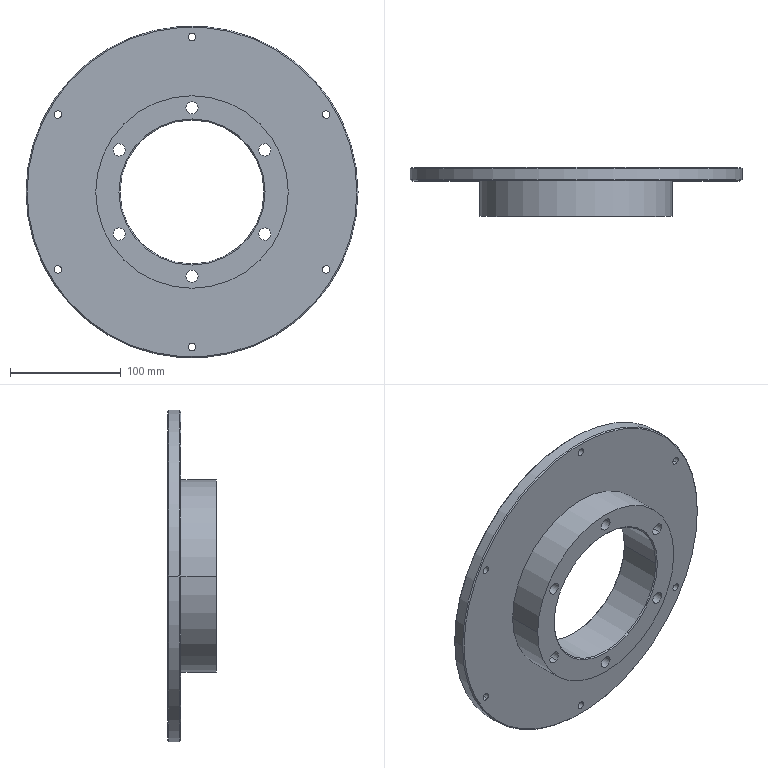Part | Creo | features CURVE 7, CUT 6, DATUM PLANE 3, PATTERN 2, CHAMFER 1, COORDINATE SYSTEM 1, PROTRUSION 1 | 1 solid | 44 faces | box 300 x 44 x 300 mm | volume 925584 mm3 | cylinder 32 | cone 8 | plane 4 | commonest cylinder face diameters 6.8 x12 11 x12 130 x2 174 x2 250 x2 300 x2
STEP:
#1=CARTESIAN_POINT('',(0.,0.,0.));
#2=DIRECTION('',(0.,0.,1.));
#3=DIRECTION('',(1.,0.,0.));
#4=AXIS2_PLACEMENT_3D('',#1,#2,#3);
#5=CARTESIAN_POINT('',(87.,0.,0.));
#6=VERTEX_POINT('',#5);
#7=CARTESIAN_POINT('',(-87.,0.,0.));
#8=VERTEX_POINT('',#7);
#9=CARTESIAN_POINT('',(0.,0.,0.));
#10=DIRECTION('',(0.,-1.,0.));
#11=DIRECTION('',(1.,0.,0.));
#12=AXIS2_PLACEMENT_3D('',#9,#10,#11);
#13=CIRCLE('',#12,87.);
#14=EDGE_CURVE('',#6,#8,#13,.T.);
#15=ORIENTED_EDGE('',*,*,#14,.F.);
#16=CARTESIAN_POINT('',(0.,0.,0.));
#17=DIRECTION('',(0.,1.,0.));
#18=DIRECTION('',(1.,0.,0.));
#19=AXIS2_PLACEMENT_3D('',#16,#17,#18);
#20=CIRCLE('',#19,87.);
#21=EDGE_CURVE('',#6,#8,#20,.T.);
#22=ORIENTED_EDGE('',*,*,#21,.T.);
#23=EDGE_LOOP('',(#15,#22));
#24=FACE_OUTER_BOUND('',#23,.F.);
#25=CARTESIAN_POINT('',(5.5,0.,-76.));
#26=VERTEX_POINT('',#25);
#27=CARTESIAN_POINT('',(-5.5,0.,-76.));
#28=VERTEX_POINT('',#27);
#29=CARTESIAN_POINT('',(0.,0.,-76.));
#30=DIRECTION('',(0.,1.,0.));
#31=DIRECTION('',(1.,0.,0.));
#32=AXIS2_PLACEMENT_3D('',#29,#30,#31);
#33=CIRCLE('',#32,5.5);
#34=EDGE_CURVE('',#26,#28,#33,.T.);
#35=ORIENTED_EDGE('',*,*,#34,.F.);
#36=CARTESIAN_POINT('',(0.,0.,-76.));
#37=DIRECTION('',(0.,1.,0.));
#38=DIRECTION('',(-1.,0.,0.));
#39=AXIS2_PLACEMENT_3D('',#36,#37,#38);
#40=CIRCLE('',#39,5.5);
#41=EDGE_CURVE('',#28,#26,#40,.T.);
#42=ORIENTED_EDGE('',*,*,#41,.F.);
#43=EDGE_LOOP('',(#35,#42));
#44=FACE_BOUND('',#43,.F.);
#45=CARTESIAN_POINT('',(-63.068,0.,-42.763));
#46=VERTEX_POINT('',#45);
#47=CARTESIAN_POINT('',(-68.568,0.,-33.237));
#48=VERTEX_POINT('',#47);
#49=CARTESIAN_POINT('',(-65.818,0.,-38.));
#50=DIRECTION('',(0.,1.,0.));
#51=DIRECTION('',(0.5,0.,-0.866));
#52=AXIS2_PLACEMENT_3D('',#49,#50,#51);
#53=CIRCLE('',#52,5.5);
#54=EDGE_CURVE('',#46,#48,#53,.T.);
#55=ORIENTED_EDGE('',*,*,#54,.F.);
#56=CARTESIAN_POINT('',(-65.818,0.,-38.));
#57=DIRECTION('',(0.,1.,0.));
#58=DIRECTION('',(-0.5,0.,0.866));
#59=AXIS2_PLACEMENT_3D('',#56,#57,#58);
#60=CIRCLE('',#59,5.5);
#61=EDGE_CURVE('',#48,#46,#60,.T.);
#62=ORIENTED_EDGE('',*,*,#61,.F.);
#63=EDGE_LOOP('',(#55,#62));
#64=FACE_BOUND('',#63,.F.);
#65=CARTESIAN_POINT('',(-68.568,0.,33.237));
#66=VERTEX_POINT('',#65);
#67=CARTESIAN_POINT('',(-63.068,0.,42.763));
#68=VERTEX_POINT('',#67);
#69=CARTESIAN_POINT('',(-65.818,0.,38.));
#70=DIRECTION('',(0.,1.,0.));
#71=DIRECTION('',(-0.5,0.,-0.866));
#72=AXIS2_PLACEMENT_3D('',#69,#70,#71);
#73=CIRCLE('',#72,5.5);
#74=EDGE_CURVE('',#66,#68,#73,.T.);
#75=ORIENTED_EDGE('',*,*,#74,.F.);
#76=CARTESIAN_POINT('',(-65.818,0.,38.));
#77=DIRECTION('',(0.,1.,0.));
#78=DIRECTION('',(0.5,0.,0.866));
#79=AXIS2_PLACEMENT_3D('',#76,#77,#78);
#80=CIRCLE('',#79,5.5);
#81=EDGE_CURVE('',#68,#66,#80,.T.);
#82=ORIENTED_EDGE('',*,*,#81,.F.);
#83=EDGE_LOOP('',(#75,#82));
#84=FACE_BOUND('',#83,.F.);
#85=CARTESIAN_POINT('',(-5.5,0.,76.));
#86=VERTEX_POINT('',#85);
#87=CARTESIAN_POINT('',(5.5,0.,76.));
#88=VERTEX_POINT('',#87);
#89=CARTESIAN_POINT('',(0.,0.,76.));
#90=DIRECTION('',(0.,1.,0.));
#91=DIRECTION('',(-1.,0.,0.));
#92=AXIS2_PLACEMENT_3D('',#89,#90,#91);
#93=CIRCLE('',#92,5.5);
#94=EDGE_CURVE('',#86,#88,#93,.T.);
#95=ORIENTED_EDGE('',*,*,#94,.F.);
#96=CARTESIAN_POINT('',(0.,0.,76.));
#97=DIRECTION('',(0.,1.,0.));
#98=DIRECTION('',(1.,0.,0.));
#99=AXIS2_PLACEMENT_3D('',#96,#97,#98);
#100=CIRCLE('',#99,5.5);
#101=EDGE_CURVE('',#88,#86,#100,.T.);
#102=ORIENTED_EDGE('',*,*,#101,.F.);
#103=EDGE_LOOP('',(#95,#102));
#104=FACE_BOUND('',#103,.F.);
#105=CARTESIAN_POINT('',(63.068,0.,42.763));
#106=VERTEX_POINT('',#105);
#107=CARTESIAN_POINT('',(68.568,0.,33.237));
#108=VERTEX_POINT('',#107);
#109=CARTESIAN_POINT('',(65.818,0.,38.));
#110=DIRECTION('',(0.,1.,0.));
#111=DIRECTION('',(-0.5,0.,0.866));
#112=AXIS2_PLACEMENT_3D('',#109,#110,#111);
#113=CIRCLE('',#112,5.5);
#114=EDGE_CURVE('',#106,#108,#113,.T.);
#115=ORIENTED_EDGE('',*,*,#114,.F.);
#116=CARTESIAN_POINT('',(65.818,0.,38.));
#117=DIRECTION('',(0.,1.,0.));
#118=DIRECTION('',(0.5,0.,-0.866));
#119=AXIS2_PLACEMENT_3D('',#116,#117,#118);
#120=CIRCLE('',#119,5.5);
#121=EDGE_CURVE('',#108,#106,#120,.T.);
#122=ORIENTED_EDGE('',*,*,#121,.F.);
#123=EDGE_LOOP('',(#115,#122));
#124=FACE_BOUND('',#123,.F.);
#125=CARTESIAN_POINT('',(68.568,0.,-33.237));
#126=VERTEX_POINT('',#125);
#127=CARTESIAN_POINT('',(63.068,0.,-42.763));
#128=VERTEX_POINT('',#127);
#129=CARTESIAN_POINT('',(65.818,0.,-38.));
#130=DIRECTION('',(0.,1.,0.));
#131=DIRECTION('',(0.5,0.,0.866));
#132=AXIS2_PLACEMENT_3D('',#129,#130,#131);
#133=CIRCLE('',#132,5.5);
#134=EDGE_CURVE('',#126,#128,#133,.T.);
#135=ORIENTED_EDGE('',*,*,#134,.F.);
#136=CARTESIAN_POINT('',(65.818,0.,-38.));
#137=DIRECTION('',(0.,1.,0.));
#138=DIRECTION('',(-0.5,0.,-0.866));
#139=AXIS2_PLACEMENT_3D('',#136,#137,#138);
#140=CIRCLE('',#139,5.5);
#141=EDGE_CURVE('',#128,#126,#140,.T.);
#142=ORIENTED_EDGE('',*,*,#141,.F.);
#143=EDGE_LOOP('',(#135,#142));
#144=FACE_BOUND('',#143,.F.);
#145=CARTESIAN_POINT('',(-66.,0.,0.));
#146=VERTEX_POINT('',#145);
#147=CARTESIAN_POINT('',(66.,0.,0.));
#148=VERTEX_POINT('',#147);
#149=CARTESIAN_POINT('',(0.,0.,0.));
#150=DIRECTION('',(0.,1.,0.));
#151=DIRECTION('',(-1.,0.,0.));
#152=AXIS2_PLACEMENT_3D('',#149,#150,#151);
#153=CIRCLE('',#152,66.);
#154=EDGE_CURVE('',#146,#148,#153,.T.);
#155=ORIENTED_EDGE('',*,*,#154,.F.);
#156=CARTESIAN_POINT('',(0.,0.,0.));
#157=DIRECTION('',(0.,1.,0.));
#158=DIRECTION('',(1.,0.,0.));
#159=AXIS2_PLACEMENT_3D('',#156,#157,#158);
#160=CIRCLE('',#159,66.);
#161=EDGE_CURVE('',#148,#146,#160,.T.);
#162=ORIENTED_EDGE('',*,*,#161,.F.);
#163=EDGE_LOOP('',(#155,#162));
#164=FACE_BOUND('',#163,.F.);
#165=CARTESIAN_POINT('',(0.,0.,0.));
#166=DIRECTION('',(0.,1.,0.));
#167=DIRECTION('',(1.,0.,0.));
#168=AXIS2_PLACEMENT_3D('',#165,#166,#167);
#169=PLANE('',#168);
#170=ADVANCED_FACE('',(#24,#44,#64,#84,#104,#124,#144,#164),#169,.F.);
#171=CARTESIAN_POINT('',(87.,32.,0.));
#172=VERTEX_POINT('',#171);
#173=CARTESIAN_POINT('',(87.,0.,0.));
#174=DIRECTION('',(0.,1.,0.));
#175=VECTOR('',#174,32.);
#176=LINE('',#173,#175);
#177=EDGE_CURVE('',#6,#172,#176,.T.);
#178=ORIENTED_EDGE('',*,*,#177,.F.);
#179=ORIENTED_EDGE('',*,*,#14,.T.);
#180=CARTESIAN_POINT('',(-87.,32.,0.));
#181=VERTEX_POINT('',#180);
#182=CARTESIAN_POINT('',(-87.,0.,0.));
#183=DIRECTION('',(0.,1.,0.));
#184=VECTOR('',#183,32.);
#185=LINE('',#182,#184);
#186=EDGE_CURVE('',#8,#181,#185,.T.);
#187=ORIENTED_EDGE('',*,*,#186,.T.);
#188=CARTESIAN_POINT('',(0.,32.,0.));
#189=DIRECTION('',(0.,-1.,0.));
#190=DIRECTION('',(1.,0.,0.));
#191=AXIS2_PLACEMENT_3D('',#188,#189,#190);
#192=CIRCLE('',#191,87.);
#193=EDGE_CURVE('',#172,#181,#192,.T.);
#194=ORIENTED_EDGE('',*,*,#193,.F.);
#195=EDGE_LOOP('',(#178,#179,#187,#194));
#196=FACE_OUTER_BOUND('',#195,.F.);
#197=CARTESIAN_POINT('',(0.,0.,0.));
#198=DIRECTION('',(0.,1.,0.));
#199=DIRECTION('',(1.,0.,0.));
#200=AXIS2_PLACEMENT_3D('',#197,#198,#199);
#201=CYLINDRICAL_SURFACE('',#200,87.);
#202=ADVANCED_FACE('',(#196),#201,.T.);
#203=ORIENTED_EDGE('',*,*,#177,.T.);
#204=CARTESIAN_POINT('',(0.,32.,0.));
#205=DIRECTION('',(0.,1.,0.));
#206=DIRECTION('',(1.,0.,0.));
#207=AXIS2_PLACEMENT_3D('',#204,#205,#206);
#208=CIRCLE('',#207,87.);
#209=EDGE_CURVE('',#172,#181,#208,.T.);
#210=ORIENTED_EDGE('',*,*,#209,.T.);
#211=ORIENTED_EDGE('',*,*,#186,.F.);
#212=ORIENTED_EDGE('',*,*,#21,.F.);
#213=EDGE_LOOP('',(#203,#210,#211,#212));
#214=FACE_OUTER_BOUND('',#213,.F.);
#215=CARTESIAN_POINT('',(0.,0.,0.));
#216=DIRECTION('',(0.,1.,0.));
#217=DIRECTION('',(1.,0.,0.));
#218=AXIS2_PLACEMENT_3D('',#215,#216,#217);
#219=CYLINDRICAL_SURFACE('',#218,87.);
#220=ADVANCED_FACE('',(#214),#219,.T.);
#221=CARTESIAN_POINT('',(-149.,32.,0.));
#222=VERTEX_POINT('',#221);
#223=CARTESIAN_POINT('',(149.,32.,0.));
#224=VERTEX_POINT('',#223);
#225=CARTESIAN_POINT('',(0.,32.,0.));
#226=DIRECTION('',(0.,1.,0.));
#227=DIRECTION('',(-1.,0.,0.));
#228=AXIS2_PLACEMENT_3D('',#225,#226,#227);
#229=CIRCLE('',#228,149.);
#230=EDGE_CURVE('',#222,#224,#229,.T.);
#231=ORIENTED_EDGE('',*,*,#230,.T.);
#232=CARTESIAN_POINT('',(0.,32.,0.));
#233=DIRECTION('',(0.,1.,0.));
#234=DIRECTION('',(1.,0.,0.));
#235=AXIS2_PLACEMENT_3D('',#232,#233,#234);
#236=CIRCLE('',#235,149.);
#237=EDGE_CURVE('',#224,#222,#236,.T.);
#238=ORIENTED_EDGE('',*,*,#237,.T.);
#239=EDGE_LOOP('',(#231,#238));
#240=FACE_OUTER_BOUND('',#239,.F.);
#241=CARTESIAN_POINT('',(3.4,32.,-140.));
#242=VERTEX_POINT('',#241);
#243=CARTESIAN_POINT('',(-3.4,32.,-140.));
#244=VERTEX_POINT('',#243);
#245=CARTESIAN_POINT('',(0.,32.,-140.));
#246=DIRECTION('',(0.,1.,0.));
#247=DIRECTION('',(1.,0.,0.));
#248=AXIS2_PLACEMENT_3D('',#245,#246,#247);
#249=CIRCLE('',#248,3.4);
#250=EDGE_CURVE('',#242,#244,#249,.T.);
#251=ORIENTED_EDGE('',*,*,#250,.F.);
#252=CARTESIAN_POINT('',(0.,32.,-140.));
#253=DIRECTION('',(0.,1.,0.));
#254=DIRECTION('',(-1.,0.,0.));
#255=AXIS2_PLACEMENT_3D('',#252,#253,#254);
#256=CIRCLE('',#255,3.4);
#257=EDGE_CURVE('',#244,#242,#256,.T.);
#258=ORIENTED_EDGE('',*,*,#257,.F.);
#259=EDGE_LOOP('',(#251,#258));
#260=FACE_BOUND('',#259,.F.);
#261=CARTESIAN_POINT('',(-119.544,32.,-72.944));
#262=VERTEX_POINT('',#261);
#263=CARTESIAN_POINT('',(-122.944,32.,-67.056));
#264=VERTEX_POINT('',#263);
#265=CARTESIAN_POINT('',(-121.244,32.,-70.));
#266=DIRECTION('',(0.,1.,0.));
#267=DIRECTION('',(0.5,0.,-0.866));
#268=AXIS2_PLACEMENT_3D('',#265,#266,#267);
#269=CIRCLE('',#268,3.4);
#270=EDGE_CURVE('',#262,#264,#269,.T.);
#271=ORIENTED_EDGE('',*,*,#270,.F.);
#272=CARTESIAN_POINT('',(-121.244,32.,-70.));
#273=DIRECTION('',(0.,1.,0.));
#274=DIRECTION('',(-0.5,0.,0.866));
#275=AXIS2_PLACEMENT_3D('',#272,#273,#274);
#276=CIRCLE('',#275,3.4);
#277=EDGE_CURVE('',#264,#262,#276,.T.);
#278=ORIENTED_EDGE('',*,*,#277,.F.);
#279=EDGE_LOOP('',(#271,#278));
#280=FACE_BOUND('',#279,.F.);
#281=CARTESIAN_POINT('',(-122.944,32.,67.056));
#282=VERTEX_POINT('',#281);
#283=CARTESIAN_POINT('',(-119.544,32.,72.944));
#284=VERTEX_POINT('',#283);
#285=CARTESIAN_POINT('',(-121.244,32.,70.));
#286=DIRECTION('',(0.,1.,0.));
#287=DIRECTION('',(-0.5,0.,-0.866));
#288=AXIS2_PLACEMENT_3D('',#285,#286,#287);
#289=CIRCLE('',#288,3.4);
#290=EDGE_CURVE('',#282,#284,#289,.T.);
#291=ORIENTED_EDGE('',*,*,#290,.F.);
#292=CARTESIAN_POINT('',(-121.244,32.,70.));
#293=DIRECTION('',(0.,1.,0.));
#294=DIRECTION('',(0.5,0.,0.866));
#295=AXIS2_PLACEMENT_3D('',#292,#293,#294);
#296=CIRCLE('',#295,3.4);
#297=EDGE_CURVE('',#284,#282,#296,.T.);
#298=ORIENTED_EDGE('',*,*,#297,.F.);
#299=EDGE_LOOP('',(#291,#298));
#300=FACE_BOUND('',#299,.F.);
#301=CARTESIAN_POINT('',(-3.4,32.,140.));
#302=VERTEX_POINT('',#301);
#303=CARTESIAN_POINT('',(3.4,32.,140.));
#304=VERTEX_POINT('',#303);
#305=CARTESIAN_POINT('',(0.,32.,140.));
#306=DIRECTION('',(0.,1.,0.));
#307=DIRECTION('',(-1.,0.,0.));
#308=AXIS2_PLACEMENT_3D('',#305,#306,#307);
#309=CIRCLE('',#308,3.4);
#310=EDGE_CURVE('',#302,#304,#309,.T.);
#311=ORIENTED_EDGE('',*,*,#310,.F.);
#312=CARTESIAN_POINT('',(0.,32.,140.));
#313=DIRECTION('',(0.,1.,0.));
#314=DIRECTION('',(1.,0.,0.));
#315=AXIS2_PLACEMENT_3D('',#312,#313,#314);
#316=CIRCLE('',#315,3.4);
#317=EDGE_CURVE('',#304,#302,#316,.T.);
#318=ORIENTED_EDGE('',*,*,#317,.F.);
#319=EDGE_LOOP('',(#311,#318));
#320=FACE_BOUND('',#319,.F.);
#321=CARTESIAN_POINT('',(119.544,32.,72.944));
#322=VERTEX_POINT('',#321);
#323=CARTESIAN_POINT('',(122.944,32.,67.056));
#324=VERTEX_POINT('',#323);
#325=CARTESIAN_POINT('',(121.244,32.,70.));
#326=DIRECTION('',(0.,1.,0.));
#327=DIRECTION('',(-0.5,0.,0.866));
#328=AXIS2_PLACEMENT_3D('',#325,#326,#327);
#329=CIRCLE('',#328,3.4);
#330=EDGE_CURVE('',#322,#324,#329,.T.);
#331=ORIENTED_EDGE('',*,*,#330,.F.);
#332=CARTESIAN_POINT('',(121.244,32.,70.));
#333=DIRECTION('',(0.,1.,0.));
#334=DIRECTION('',(0.5,0.,-0.866));
#335=AXIS2_PLACEMENT_3D('',#332,#333,#334);
#336=CIRCLE('',#335,3.4);
#337=EDGE_CURVE('',#324,#322,#336,.T.);
#338=ORIENTED_EDGE('',*,*,#337,.F.);
#339=EDGE_LOOP('',(#331,#338));
#340=FACE_BOUND('',#339,.F.);
#341=CARTESIAN_POINT('',(122.944,32.,-67.056));
#342=VERTEX_POINT('',#341);
#343=CARTESIAN_POINT('',(119.544,32.,-72.944));
#344=VERTEX_POINT('',#343);
#345=CARTESIAN_POINT('',(121.244,32.,-70.));
#346=DIRECTION('',(0.,1.,0.));
#347=DIRECTION('',(0.5,0.,0.866));
#348=AXIS2_PLACEMENT_3D('',#345,#346,#347);
#349=CIRCLE('',#348,3.4);
#350=EDGE_CURVE('',#342,#344,#349,.T.);
#351=ORIENTED_EDGE('',*,*,#350,.F.);
#352=CARTESIAN_POINT('',(121.244,32.,-70.));
#353=DIRECTION('',(0.,1.,0.));
#354=DIRECTION('',(-0.5,0.,-0.866));
#355=AXIS2_PLACEMENT_3D('',#352,#353,#354);
#356=CIRCLE('',#355,3.4);
#357=EDGE_CURVE('',#344,#342,#356,.T.);
#358=ORIENTED_EDGE('',*,*,#357,.F.);
#359=EDGE_LOOP('',(#351,#358));
#360=FACE_BOUND('',#359,.F.);
#361=ORIENTED_EDGE('',*,*,#209,.F.);
#362=ORIENTED_EDGE('',*,*,#193,.T.);
#363=EDGE_LOOP('',(#361,#362));
#364=FACE_BOUND('',#363,.F.);
#365=CARTESIAN_POINT('',(0.,32.,0.));
#366=DIRECTION('',(0.,1.,0.));
#367=DIRECTION('',(1.,0.,0.));
#368=AXIS2_PLACEMENT_3D('',#365,#366,#367);
#369=PLANE('',#368);
#370=ADVANCED_FACE('',(#240,#260,#280,#300,#320,#340,#360,#364),#369,.F.);
#371=ORIENTED_EDGE('',*,*,#250,.T.);
#372=CARTESIAN_POINT('',(-3.4,44.,-140.));
#373=VERTEX_POINT('',#372);
#374=CARTESIAN_POINT('',(-3.4,44.,-140.));
#375=DIRECTION('',(0.,-1.,0.));
#376=VECTOR('',#375,12.);
#377=LINE('',#374,#376);
#378=EDGE_CURVE('',#373,#244,#377,.T.);
#379=ORIENTED_EDGE('',*,*,#378,.F.);
#380=CARTESIAN_POINT('',(3.4,44.,-140.));
#381=VERTEX_POINT('',#380);
#382=CARTESIAN_POINT('',(0.,44.,-140.));
#383=DIRECTION('',(0.,1.,0.));
#384=DIRECTION('',(1.,0.,0.));
#385=AXIS2_PLACEMENT_3D('',#382,#383,#384);
#386=CIRCLE('',#385,3.4);
#387=EDGE_CURVE('',#381,#373,#386,.T.);
#388=ORIENTED_EDGE('',*,*,#387,.F.);
#389=CARTESIAN_POINT('',(3.4,44.,-140.));
#390=DIRECTION('',(0.,-1.,0.));
#391=VECTOR('',#390,12.);
#392=LINE('',#389,#391);
#393=EDGE_CURVE('',#381,#242,#392,.T.);
#394=ORIENTED_EDGE('',*,*,#393,.T.);
#395=EDGE_LOOP('',(#371,#379,#388,#394));
#396=FACE_OUTER_BOUND('',#395,.F.);
#397=CARTESIAN_POINT('',(0.,44.,-140.));
#398=DIRECTION('',(0.,1.,0.));
#399=DIRECTION('',(1.,0.,0.));
#400=AXIS2_PLACEMENT_3D('',#397,#398,#399);
#401=CYLINDRICAL_SURFACE('',#400,3.4);
#402=ADVANCED_FACE('',(#396),#401,.F.);
#403=ORIENTED_EDGE('',*,*,#257,.T.);
#404=ORIENTED_EDGE('',*,*,#393,.F.);
#405=CARTESIAN_POINT('',(0.,44.,-140.));
#406=DIRECTION('',(0.,1.,0.));
#407=DIRECTION('',(-1.,0.,0.));
#408=AXIS2_PLACEMENT_3D('',#405,#406,#407);
#409=CIRCLE('',#408,3.4);
#410=EDGE_CURVE('',#373,#381,#409,.T.);
#411=ORIENTED_EDGE('',*,*,#410,.F.);
#412=ORIENTED_EDGE('',*,*,#378,.T.);
#413=EDGE_LOOP('',(#403,#404,#411,#412));
#414=FACE_OUTER_BOUND('',#413,.F.);
#415=CARTESIAN_POINT('',(0.,44.,-140.));
#416=DIRECTION('',(0.,1.,0.));
#417=DIRECTION('',(1.,0.,0.));
#418=AXIS2_PLACEMENT_3D('',#415,#416,#417);
#419=CYLINDRICAL_SURFACE('',#418,3.4);
#420=ADVANCED_FACE('',(#414),#419,.F.);
#421=CARTESIAN_POINT('',(-149.,44.,0.));
#422=VERTEX_POINT('',#421);
#423=CARTESIAN_POINT('',(149.,44.,0.));
#424=VERTEX_POINT('',#423);
#425=CARTESIAN_POINT('',(0.,44.,0.));
#426=DIRECTION('',(0.,1.,0.));
#427=DIRECTION('',(-1.,0.,0.));
#428=AXIS2_PLACEMENT_3D('',#425,#426,#427);
#429=CIRCLE('',#428,149.);
#430=EDGE_CURVE('',#422,#424,#429,.T.);
#431=ORIENTED_EDGE('',*,*,#430,.F.);
#432=CARTESIAN_POINT('',(0.,44.,0.));
#433=DIRECTION('',(0.,1.,0.));
#434=DIRECTION('',(1.,0.,0.));
#435=AXIS2_PLACEMENT_3D('',#432,#433,#434);
#436=CIRCLE('',#435,149.);
#437=EDGE_CURVE('',#424,#422,#436,.T.);
#438=ORIENTED_EDGE('',*,*,#437,.F.);
#439=EDGE_LOOP('',(#431,#438));
#440=FACE_OUTER_BOUND('',#439,.F.);
#441=ORIENTED_EDGE('',*,*,#387,.T.);
#442=ORIENTED_EDGE('',*,*,#410,.T.);
#443=EDGE_LOOP('',(#441,#442));
#444=FACE_BOUND('',#443,.F.);
#445=CARTESIAN_POINT('',(-119.544,44.,-72.944));
#446=VERTEX_POINT('',#445);
#447=CARTESIAN_POINT('',(-122.944,44.,-67.056));
#448=VERTEX_POINT('',#447);
#449=CARTESIAN_POINT('',(-121.244,44.,-70.));
#450=DIRECTION('',(0.,1.,0.));
#451=DIRECTION('',(0.5,0.,-0.866));
#452=AXIS2_PLACEMENT_3D('',#449,#450,#451);
#453=CIRCLE('',#452,3.4);
#454=EDGE_CURVE('',#446,#448,#453,.T.);
#455=ORIENTED_EDGE('',*,*,#454,.T.);
#456=CARTESIAN_POINT('',(-121.244,44.,-70.));
#457=DIRECTION('',(0.,1.,0.));
#458=DIRECTION('',(-0.5,0.,0.866));
#459=AXIS2_PLACEMENT_3D('',#456,#457,#458);
#460=CIRCLE('',#459,3.4);
#461=EDGE_CURVE('',#448,#446,#460,.T.);
#462=ORIENTED_EDGE('',*,*,#461,.T.);
#463=EDGE_LOOP('',(#455,#462));
#464=FACE_BOUND('',#463,.F.);
#465=CARTESIAN_POINT('',(-122.944,44.,67.056));
#466=VERTEX_POINT('',#465);
#467=CARTESIAN_POINT('',(-119.544,44.,72.944));
#468=VERTEX_POINT('',#467);
#469=CARTESIAN_POINT('',(-121.244,44.,70.));
#470=DIRECTION('',(0.,1.,0.));
#471=DIRECTION('',(-0.5,0.,-0.866));
#472=AXIS2_PLACEMENT_3D('',#469,#470,#471);
#473=CIRCLE('',#472,3.4);
#474=EDGE_CURVE('',#466,#468,#473,.T.);
#475=ORIENTED_EDGE('',*,*,#474,.T.);
#476=CARTESIAN_POINT('',(-121.244,44.,70.));
#477=DIRECTION('',(0.,1.,0.));
#478=DIRECTION('',(0.5,0.,0.866));
#479=AXIS2_PLACEMENT_3D('',#476,#477,#478);
#480=CIRCLE('',#479,3.4);
#481=EDGE_CURVE('',#468,#466,#480,.T.);
#482=ORIENTED_EDGE('',*,*,#481,.T.);
#483=EDGE_LOOP('',(#475,#482));
#484=FACE_BOUND('',#483,.F.);
#485=CARTESIAN_POINT('',(-3.4,44.,140.));
#486=VERTEX_POINT('',#485);
#487=CARTESIAN_POINT('',(3.4,44.,140.));
#488=VERTEX_POINT('',#487);
#489=CARTESIAN_POINT('',(0.,44.,140.));
#490=DIRECTION('',(0.,1.,0.));
#491=DIRECTION('',(-1.,0.,0.));
#492=AXIS2_PLACEMENT_3D('',#489,#490,#491);
#493=CIRCLE('',#492,3.4);
#494=EDGE_CURVE('',#486,#488,#493,.T.);
#495=ORIENTED_EDGE('',*,*,#494,.T.);
#496=CARTESIAN_POINT('',(0.,44.,140.));
#497=DIRECTION('',(0.,1.,0.));
#498=DIRECTION('',(1.,0.,0.));
#499=AXIS2_PLACEMENT_3D('',#496,#497,#498);
#500=CIRCLE('',#499,3.4);
#501=EDGE_CURVE('',#488,#486,#500,.T.);
#502=ORIENTED_EDGE('',*,*,#501,.T.);
#503=EDGE_LOOP('',(#495,#502));
#504=FACE_BOUND('',#503,.F.);
#505=CARTESIAN_POINT('',(119.544,44.,72.944));
#506=VERTEX_POINT('',#505);
#507=CARTESIAN_POINT('',(122.944,44.,67.056));
#508=VERTEX_POINT('',#507);
#509=CARTESIAN_POINT('',(121.244,44.,70.));
#510=DIRECTION('',(0.,1.,0.));
#511=DIRECTION('',(-0.5,0.,0.866));
#512=AXIS2_PLACEMENT_3D('',#509,#510,#511);
#513=CIRCLE('',#512,3.4);
#514=EDGE_CURVE('',#506,#508,#513,.T.);
#515=ORIENTED_EDGE('',*,*,#514,.T.);
#516=CARTESIAN_POINT('',(121.244,44.,70.));
#517=DIRECTION('',(0.,1.,0.));
#518=DIRECTION('',(0.5,0.,-0.866));
#519=AXIS2_PLACEMENT_3D('',#516,#517,#518);
#520=CIRCLE('',#519,3.4);
#521=EDGE_CURVE('',#508,#506,#520,.T.);
#522=ORIENTED_EDGE('',*,*,#521,.T.);
#523=EDGE_LOOP('',(#515,#522));
#524=FACE_BOUND('',#523,.F.);
#525=CARTESIAN_POINT('',(122.944,44.,-67.056));
#526=VERTEX_POINT('',#525);
#527=CARTESIAN_POINT('',(119.544,44.,-72.944));
#528=VERTEX_POINT('',#527);
#529=CARTESIAN_POINT('',(121.244,44.,-70.));
#530=DIRECTION('',(0.,1.,0.));
#531=DIRECTION('',(0.5,0.,0.866));
#532=AXIS2_PLACEMENT_3D('',#529,#530,#531);
#533=CIRCLE('',#532,3.4);
#534=EDGE_CURVE('',#526,#528,#533,.T.);
#535=ORIENTED_EDGE('',*,*,#534,.T.);
#536=CARTESIAN_POINT('',(121.244,44.,-70.));
#537=DIRECTION('',(0.,1.,0.));
#538=DIRECTION('',(-0.5,0.,-0.866));
#539=AXIS2_PLACEMENT_3D('',#536,#537,#538);
#540=CIRCLE('',#539,3.4);
#541=EDGE_CURVE('',#528,#526,#540,.T.);
#542=ORIENTED_EDGE('',*,*,#541,.T.);
#543=EDGE_LOOP('',(#535,#542));
#544=FACE_BOUND('',#543,.F.);
#545=CARTESIAN_POINT('',(125.,44.,0.));
#546=VERTEX_POINT('',#545);
#547=CARTESIAN_POINT('',(-125.,44.,0.));
#548=VERTEX_POINT('',#547);
#549=CARTESIAN_POINT('',(0.,44.,0.));
#550=DIRECTION('',(0.,-1.,0.));
#551=DIRECTION('',(1.,0.,0.));
#552=AXIS2_PLACEMENT_3D('',#549,#550,#551);
#553=CIRCLE('',#552,125.);
#554=EDGE_CURVE('',#546,#548,#553,.T.);
#555=ORIENTED_EDGE('',*,*,#554,.F.);
#556=CARTESIAN_POINT('',(0.,44.,0.));
#557=DIRECTION('',(0.,1.,0.));
#558=DIRECTION('',(1.,0.,0.));
#559=AXIS2_PLACEMENT_3D('',#556,#557,#558);
#560=CIRCLE('',#559,125.);
#561=EDGE_CURVE('',#546,#548,#560,.T.);
#562=ORIENTED_EDGE('',*,*,#561,.T.);
#563=EDGE_LOOP('',(#555,#562));
#564=FACE_BOUND('',#563,.F.);
#565=CARTESIAN_POINT('',(0.,44.,0.));
#566=DIRECTION('',(0.,1.,0.));
#567=DIRECTION('',(1.,0.,0.));
#568=AXIS2_PLACEMENT_3D('',#565,#566,#567);
#569=PLANE('',#568);
#570=ADVANCED_FACE('',(#440,#444,#464,#484,#504,#524,#544,#564),#569,.T.);
#571=CARTESIAN_POINT('',(125.,42.,0.));
#572=VERTEX_POINT('',#571);
#573=CARTESIAN_POINT('',(125.,44.,0.));
#574=DIRECTION('',(0.,-1.,0.));
#575=VECTOR('',#574,2.);
#576=LINE('',#573,#575);
#577=EDGE_CURVE('',#546,#572,#576,.T.);
#578=ORIENTED_EDGE('',*,*,#577,.F.);
#579=ORIENTED_EDGE('',*,*,#554,.T.);
#580=CARTESIAN_POINT('',(-125.,42.,0.));
#581=VERTEX_POINT('',#580);
#582=CARTESIAN_POINT('',(-125.,44.,0.));
#583=DIRECTION('',(0.,-1.,0.));
#584=VECTOR('',#583,2.);
#585=LINE('',#582,#584);
#586=EDGE_CURVE('',#548,#581,#585,.T.);
#587=ORIENTED_EDGE('',*,*,#586,.T.);
#588=CARTESIAN_POINT('',(0.,42.,0.));
#589=DIRECTION('',(0.,-1.,0.));
#590=DIRECTION('',(1.,0.,0.));
#591=AXIS2_PLACEMENT_3D('',#588,#589,#590);
#592=CIRCLE('',#591,125.);
#593=EDGE_CURVE('',#572,#581,#592,.T.);
#594=ORIENTED_EDGE('',*,*,#593,.F.);
#595=EDGE_LOOP('',(#578,#579,#587,#594));
#596=FACE_OUTER_BOUND('',#595,.F.);
#597=CARTESIAN_POINT('',(0.,0.,0.));
#598=DIRECTION('',(0.,1.,0.));
#599=DIRECTION('',(1.,0.,0.));
#600=AXIS2_PLACEMENT_3D('',#597,#598,#599);
#601=CYLINDRICAL_SURFACE('',#600,125.);
#602=ADVANCED_FACE('',(#596),#601,.F.);
#603=ORIENTED_EDGE('',*,*,#577,.T.);
#604=CARTESIAN_POINT('',(0.,42.,0.));
#605=DIRECTION('',(0.,1.,0.));
#606=DIRECTION('',(1.,0.,0.));
#607=AXIS2_PLACEMENT_3D('',#604,#605,#606);
#608=CIRCLE('',#607,125.);
#609=EDGE_CURVE('',#572,#581,#608,.T.);
#610=ORIENTED_EDGE('',*,*,#609,.T.);
#611=ORIENTED_EDGE('',*,*,#586,.F.);
#612=ORIENTED_EDGE('',*,*,#561,.F.);
#613=EDGE_LOOP('',(#603,#610,#611,#612));
#614=FACE_OUTER_BOUND('',#613,.F.);
#615=CARTESIAN_POINT('',(0.,0.,0.));
#616=DIRECTION('',(0.,1.,0.));
#617=DIRECTION('',(1.,0.,0.));
#618=AXIS2_PLACEMENT_3D('',#615,#616,#617);
#619=CYLINDRICAL_SURFACE('',#618,125.);
#620=ADVANCED_FACE('',(#614),#619,.F.);
#621=ORIENTED_EDGE('',*,*,#609,.F.);
#622=ORIENTED_EDGE('',*,*,#593,.T.);
#623=EDGE_LOOP('',(#621,#622));
#624=FACE_OUTER_BOUND('',#623,.F.);
#625=CARTESIAN_POINT('',(5.5,42.,-76.));
#626=VERTEX_POINT('',#625);
#627=CARTESIAN_POINT('',(-5.5,42.,-76.));
#628=VERTEX_POINT('',#627);
#629=CARTESIAN_POINT('',(0.,42.,-76.));
#630=DIRECTION('',(0.,1.,0.));
#631=DIRECTION('',(1.,0.,0.));
#632=AXIS2_PLACEMENT_3D('',#629,#630,#631);
#633=CIRCLE('',#632,5.5);
#634=EDGE_CURVE('',#626,#628,#633,.T.);
#635=ORIENTED_EDGE('',*,*,#634,.T.);
#636=CARTESIAN_POINT('',(0.,42.,-76.));
#637=DIRECTION('',(0.,1.,0.));
#638=DIRECTION('',(-1.,0.,0.));
#639=AXIS2_PLACEMENT_3D('',#636,#637,#638);
#640=CIRCLE('',#639,5.5);
#641=EDGE_CURVE('',#628,#626,#640,.T.);
#642=ORIENTED_EDGE('',*,*,#641,.T.);
#643=EDGE_LOOP('',(#635,#642));
#644=FACE_BOUND('',#643,.F.);
#645=CARTESIAN_POINT('',(-63.068,42.,-42.763));
#646=VERTEX_POINT('',#645);
#647=CARTESIAN_POINT('',(-68.568,42.,-33.237));
#648=VERTEX_POINT('',#647);
#649=CARTESIAN_POINT('',(-65.818,42.,-38.));
#650=DIRECTION('',(0.,1.,0.));
#651=DIRECTION('',(0.5,0.,-0.866));
#652=AXIS2_PLACEMENT_3D('',#649,#650,#651);
#653=CIRCLE('',#652,5.5);
#654=EDGE_CURVE('',#646,#648,#653,.T.);
#655=ORIENTED_EDGE('',*,*,#654,.T.);
#656=CARTESIAN_POINT('',(-65.818,42.,-38.));
#657=DIRECTION('',(0.,1.,0.));
#658=DIRECTION('',(-0.5,0.,0.866));
#659=AXIS2_PLACEMENT_3D('',#656,#657,#658);
#660=CIRCLE('',#659,5.5);
#661=EDGE_CURVE('',#648,#646,#660,.T.);
#662=ORIENTED_EDGE('',*,*,#661,.T.);
#663=EDGE_LOOP('',(#655,#662));
#664=FACE_BOUND('',#663,.F.);
#665=CARTESIAN_POINT('',(-68.568,42.,33.237));
#666=VERTEX_POINT('',#665);
#667=CARTESIAN_POINT('',(-63.068,42.,42.763));
#668=VERTEX_POINT('',#667);
#669=CARTESIAN_POINT('',(-65.818,42.,38.));
#670=DIRECTION('',(0.,1.,0.));
#671=DIRECTION('',(-0.5,0.,-0.866));
#672=AXIS2_PLACEMENT_3D('',#669,#670,#671);
#673=CIRCLE('',#672,5.5);
#674=EDGE_CURVE('',#666,#668,#673,.T.);
#675=ORIENTED_EDGE('',*,*,#674,.T.);
#676=CARTESIAN_POINT('',(-65.818,42.,38.));
#677=DIRECTION('',(0.,1.,0.));
#678=DIRECTION('',(0.5,0.,0.866));
#679=AXIS2_PLACEMENT_3D('',#676,#677,#678);
#680=CIRCLE('',#679,5.5);
#681=EDGE_CURVE('',#668,#666,#680,.T.);
#682=ORIENTED_EDGE('',*,*,#681,.T.);
#683=EDGE_LOOP('',(#675,#682));
#684=FACE_BOUND('',#683,.F.);
#685=CARTESIAN_POINT('',(-5.5,42.,76.));
#686=VERTEX_POINT('',#685);
#687=CARTESIAN_POINT('',(5.5,42.,76.));
#688=VERTEX_POINT('',#687);
#689=CARTESIAN_POINT('',(0.,42.,76.));
#690=DIRECTION('',(0.,1.,0.));
#691=DIRECTION('',(-1.,0.,0.));
#692=AXIS2_PLACEMENT_3D('',#689,#690,#691);
#693=CIRCLE('',#692,5.5);
#694=EDGE_CURVE('',#686,#688,#693,.T.);
#695=ORIENTED_EDGE('',*,*,#694,.T.);
#696=CARTESIAN_POINT('',(0.,42.,76.));
#697=DIRECTION('',(0.,1.,0.));
#698=DIRECTION('',(1.,0.,0.));
#699=AXIS2_PLACEMENT_3D('',#696,#697,#698);
#700=CIRCLE('',#699,5.5);
#701=EDGE_CURVE('',#688,#686,#700,.T.);
#702=ORIENTED_EDGE('',*,*,#701,.T.);
#703=EDGE_LOOP('',(#695,#702));
#704=FACE_BOUND('',#703,.F.);
#705=CARTESIAN_POINT('',(63.068,42.,42.763));
#706=VERTEX_POINT('',#705);
#707=CARTESIAN_POINT('',(68.568,42.,33.237));
#708=VERTEX_POINT('',#707);
#709=CARTESIAN_POINT('',(65.818,42.,38.));
#710=DIRECTION('',(0.,1.,0.));
#711=DIRECTION('',(-0.5,0.,0.866));
#712=AXIS2_PLACEMENT_3D('',#709,#710,#711);
#713=CIRCLE('',#712,5.5);
#714=EDGE_CURVE('',#706,#708,#713,.T.);
#715=ORIENTED_EDGE('',*,*,#714,.T.);
#716=CARTESIAN_POINT('',(65.818,42.,38.));
#717=DIRECTION('',(0.,1.,0.));
#718=DIRECTION('',(0.5,0.,-0.866));
#719=AXIS2_PLACEMENT_3D('',#716,#717,#718);
#720=CIRCLE('',#719,5.5);
#721=EDGE_CURVE('',#708,#706,#720,.T.);
#722=ORIENTED_EDGE('',*,*,#721,.T.);
#723=EDGE_LOOP('',(#715,#722));
#724=FACE_BOUND('',#723,.F.);
#725=CARTESIAN_POINT('',(68.568,42.,-33.237));
#726=VERTEX_POINT('',#725);
#727=CARTESIAN_POINT('',(63.068,42.,-42.763));
#728=VERTEX_POINT('',#727);
#729=CARTESIAN_POINT('',(65.818,42.,-38.));
#730=DIRECTION('',(0.,1.,0.));
#731=DIRECTION('',(0.5,0.,0.866));
#732=AXIS2_PLACEMENT_3D('',#729,#730,#731);
#733=CIRCLE('',#732,5.5);
#734=EDGE_CURVE('',#726,#728,#733,.T.);
#735=ORIENTED_EDGE('',*,*,#734,.T.);
#736=CARTESIAN_POINT('',(65.818,42.,-38.));
#737=DIRECTION('',(0.,1.,0.));
#738=DIRECTION('',(-0.5,0.,-0.866));
#739=AXIS2_PLACEMENT_3D('',#736,#737,#738);
#740=CIRCLE('',#739,5.5);
#741=EDGE_CURVE('',#728,#726,#740,.T.);
#742=ORIENTED_EDGE('',*,*,#741,.T.);
#743=EDGE_LOOP('',(#735,#742));
#744=FACE_BOUND('',#743,.F.);
#745=CARTESIAN_POINT('',(-66.,42.,0.));
#746=VERTEX_POINT('',#745);
#747=CARTESIAN_POINT('',(66.,42.,0.));
#748=VERTEX_POINT('',#747);
#749=CARTESIAN_POINT('',(0.,42.,0.));
#750=DIRECTION('',(0.,1.,0.));
#751=DIRECTION('',(-1.,0.,0.));
#752=AXIS2_PLACEMENT_3D('',#749,#750,#751);
#753=CIRCLE('',#752,66.);
#754=EDGE_CURVE('',#746,#748,#753,.T.);
#755=ORIENTED_EDGE('',*,*,#754,.T.);
#756=CARTESIAN_POINT('',(0.,42.,0.));
#757=DIRECTION('',(0.,1.,0.));
#758=DIRECTION('',(1.,0.,0.));
#759=AXIS2_PLACEMENT_3D('',#756,#757,#758);
#760=CIRCLE('',#759,66.);
#761=EDGE_CURVE('',#748,#746,#760,.T.);
#762=ORIENTED_EDGE('',*,*,#761,.T.);
#763=EDGE_LOOP('',(#755,#762));
#764=FACE_BOUND('',#763,.F.);
#765=CARTESIAN_POINT('',(0.,42.,0.));
#766=DIRECTION('',(0.,1.,0.));
#767=DIRECTION('',(1.,0.,0.));
#768=AXIS2_PLACEMENT_3D('',#765,#766,#767);
#769=PLANE('',#768);
#770=ADVANCED_FACE('',(#624,#644,#664,#684,#704,#724,#744,#764),#769,.T.);
#771=ORIENTED_EDGE('',*,*,#34,.T.);
#772=CARTESIAN_POINT('',(-5.5,42.,-76.));
#773=DIRECTION('',(0.,-1.,0.));
#774=VECTOR('',#773,42.);
#775=LINE('',#772,#774);
#776=EDGE_CURVE('',#628,#28,#775,.T.);
#777=ORIENTED_EDGE('',*,*,#776,.F.);
#778=ORIENTED_EDGE('',*,*,#634,.F.);
#779=CARTESIAN_POINT('',(5.5,42.,-76.));
#780=DIRECTION('',(0.,-1.,0.));
#781=VECTOR('',#780,42.);
#782=LINE('',#779,#781);
#783=EDGE_CURVE('',#626,#26,#782,.T.);
#784=ORIENTED_EDGE('',*,*,#783,.T.);
#785=EDGE_LOOP('',(#771,#777,#778,#784));
#786=FACE_OUTER_BOUND('',#785,.F.);
#787=CARTESIAN_POINT('',(0.,44.,-76.));
#788=DIRECTION('',(0.,1.,0.));
#789=DIRECTION('',(1.,0.,0.));
#790=AXIS2_PLACEMENT_3D('',#787,#788,#789);
#791=CYLINDRICAL_SURFACE('',#790,5.5);
#792=ADVANCED_FACE('',(#786),#791,.F.);
#793=ORIENTED_EDGE('',*,*,#41,.T.);
#794=ORIENTED_EDGE('',*,*,#783,.F.);
#795=ORIENTED_EDGE('',*,*,#641,.F.);
#796=ORIENTED_EDGE('',*,*,#776,.T.);
#797=EDGE_LOOP('',(#793,#794,#795,#796));
#798=FACE_OUTER_BOUND('',#797,.F.);
#799=CARTESIAN_POINT('',(0.,44.,-76.));
#800=DIRECTION('',(0.,1.,0.));
#801=DIRECTION('',(1.,0.,0.));
#802=AXIS2_PLACEMENT_3D('',#799,#800,#801);
#803=CYLINDRICAL_SURFACE('',#802,5.5);
#804=ADVANCED_FACE('',(#798),#803,.F.);
#805=ORIENTED_EDGE('',*,*,#54,.T.);
#806=CARTESIAN_POINT('',(-68.568,42.,-33.237));
#807=DIRECTION('',(0.,-1.,0.));
#808=VECTOR('',#807,42.);
#809=LINE('',#806,#808);
#810=EDGE_CURVE('',#648,#48,#809,.T.);
#811=ORIENTED_EDGE('',*,*,#810,.F.);
#812=ORIENTED_EDGE('',*,*,#654,.F.);
#813=CARTESIAN_POINT('',(-63.068,42.,-42.763));
#814=DIRECTION('',(0.,-1.,0.));
#815=VECTOR('',#814,42.);
#816=LINE('',#813,#815);
#817=EDGE_CURVE('',#646,#46,#816,.T.);
#818=ORIENTED_EDGE('',*,*,#817,.T.);
#819=EDGE_LOOP('',(#805,#811,#812,#818));
#820=FACE_OUTER_BOUND('',#819,.F.);
#821=CARTESIAN_POINT('',(-65.818,44.,-38.));
#822=DIRECTION('',(0.,1.,0.));
#823=DIRECTION('',(0.5,0.,-0.866));
#824=AXIS2_PLACEMENT_3D('',#821,#822,#823);
#825=CYLINDRICAL_SURFACE('',#824,5.5);
#826=ADVANCED_FACE('',(#820),#825,.F.);
#827=ORIENTED_EDGE('',*,*,#61,.T.);
#828=ORIENTED_EDGE('',*,*,#817,.F.);
#829=ORIENTED_EDGE('',*,*,#661,.F.);
#830=ORIENTED_EDGE('',*,*,#810,.T.);
#831=EDGE_LOOP('',(#827,#828,#829,#830));
#832=FACE_OUTER_BOUND('',#831,.F.);
#833=CARTESIAN_POINT('',(-65.818,44.,-38.));
#834=DIRECTION('',(0.,1.,0.));
#835=DIRECTION('',(0.5,0.,-0.866));
#836=AXIS2_PLACEMENT_3D('',#833,#834,#835);
#837=CYLINDRICAL_SURFACE('',#836,5.5);
#838=ADVANCED_FACE('',(#832),#837,.F.);
#839=ORIENTED_EDGE('',*,*,#74,.T.);
#840=CARTESIAN_POINT('',(-63.068,42.,42.763));
#841=DIRECTION('',(0.,-1.,0.));
#842=VECTOR('',#841,42.);
#843=LINE('',#840,#842);
#844=EDGE_CURVE('',#668,#68,#843,.T.);
#845=ORIENTED_EDGE('',*,*,#844,.F.);
#846=ORIENTED_EDGE('',*,*,#674,.F.);
#847=CARTESIAN_POINT('',(-68.568,42.,33.237));
#848=DIRECTION('',(0.,-1.,0.));
#849=VECTOR('',#848,42.);
#850=LINE('',#847,#849);
#851=EDGE_CURVE('',#666,#66,#850,.T.);
#852=ORIENTED_EDGE('',*,*,#851,.T.);
#853=EDGE_LOOP('',(#839,#845,#846,#852));
#854=FACE_OUTER_BOUND('',#853,.F.);
#855=CARTESIAN_POINT('',(-65.818,44.,38.));
#856=DIRECTION('',(0.,1.,0.));
#857=DIRECTION('',(-0.5,0.,-0.866));
#858=AXIS2_PLACEMENT_3D('',#855,#856,#857);
#859=CYLINDRICAL_SURFACE('',#858,5.5);
#860=ADVANCED_FACE('',(#854),#859,.F.);
#861=ORIENTED_EDGE('',*,*,#81,.T.);
#862=ORIENTED_EDGE('',*,*,#851,.F.);
#863=ORIENTED_EDGE('',*,*,#681,.F.);
#864=ORIENTED_EDGE('',*,*,#844,.T.);
#865=EDGE_LOOP('',(#861,#862,#863,#864));
#866=FACE_OUTER_BOUND('',#865,.F.);
#867=CARTESIAN_POINT('',(-65.818,44.,38.));
#868=DIRECTION('',(0.,1.,0.));
#869=DIRECTION('',(-0.5,0.,-0.866));
#870=AXIS2_PLACEMENT_3D('',#867,#868,#869);
#871=CYLINDRICAL_SURFACE('',#870,5.5);
#872=ADVANCED_FACE('',(#866),#871,.F.);
#873=ORIENTED_EDGE('',*,*,#94,.T.);
#874=CARTESIAN_POINT('',(5.5,42.,76.));
#875=DIRECTION('',(0.,-1.,0.));
#876=VECTOR('',#875,42.);
#877=LINE('',#874,#876);
#878=EDGE_CURVE('',#688,#88,#877,.T.);
#879=ORIENTED_EDGE('',*,*,#878,.F.);
#880=ORIENTED_EDGE('',*,*,#694,.F.);
#881=CARTESIAN_POINT('',(-5.5,42.,76.));
#882=DIRECTION('',(0.,-1.,0.));
#883=VECTOR('',#882,42.);
#884=LINE('',#881,#883);
#885=EDGE_CURVE('',#686,#86,#884,.T.);
#886=ORIENTED_EDGE('',*,*,#885,.T.);
#887=EDGE_LOOP('',(#873,#879,#880,#886));
#888=FACE_OUTER_BOUND('',#887,.F.);
#889=CARTESIAN_POINT('',(0.,44.,76.));
#890=DIRECTION('',(0.,1.,0.));
#891=DIRECTION('',(-1.,0.,0.));
#892=AXIS2_PLACEMENT_3D('',#889,#890,#891);
#893=CYLINDRICAL_SURFACE('',#892,5.5);
#894=ADVANCED_FACE('',(#888),#893,.F.);
#895=ORIENTED_EDGE('',*,*,#101,.T.);
#896=ORIENTED_EDGE('',*,*,#885,.F.);
#897=ORIENTED_EDGE('',*,*,#701,.F.);
#898=ORIENTED_EDGE('',*,*,#878,.T.);
#899=EDGE_LOOP('',(#895,#896,#897,#898));
#900=FACE_OUTER_BOUND('',#899,.F.);
#901=CARTESIAN_POINT('',(0.,44.,76.));
#902=DIRECTION('',(0.,1.,0.));
#903=DIRECTION('',(-1.,0.,0.));
#904=AXIS2_PLACEMENT_3D('',#901,#902,#903);
#905=CYLINDRICAL_SURFACE('',#904,5.5);
#906=ADVANCED_FACE('',(#900),#905,.F.);
#907=ORIENTED_EDGE('',*,*,#114,.T.);
#908=CARTESIAN_POINT('',(68.568,42.,33.237));
#909=DIRECTION('',(0.,-1.,0.));
#910=VECTOR('',#909,42.);
#911=LINE('',#908,#910);
#912=EDGE_CURVE('',#708,#108,#911,.T.);
#913=ORIENTED_EDGE('',*,*,#912,.F.);
#914=ORIENTED_EDGE('',*,*,#714,.F.);
#915=CARTESIAN_POINT('',(63.068,42.,42.763));
#916=DIRECTION('',(0.,-1.,0.));
#917=VECTOR('',#916,42.);
#918=LINE('',#915,#917);
#919=EDGE_CURVE('',#706,#106,#918,.T.);
#920=ORIENTED_EDGE('',*,*,#919,.T.);
#921=EDGE_LOOP('',(#907,#913,#914,#920));
#922=FACE_OUTER_BOUND('',#921,.F.);
#923=CARTESIAN_POINT('',(65.818,44.,38.));
#924=DIRECTION('',(0.,1.,0.));
#925=DIRECTION('',(-0.5,0.,0.866));
#926=AXIS2_PLACEMENT_3D('',#923,#924,#925);
#927=CYLINDRICAL_SURFACE('',#926,5.5);
#928=ADVANCED_FACE('',(#922),#927,.F.);
#929=ORIENTED_EDGE('',*,*,#121,.T.);
#930=ORIENTED_EDGE('',*,*,#919,.F.);
#931=ORIENTED_EDGE('',*,*,#721,.F.);
#932=ORIENTED_EDGE('',*,*,#912,.T.);
#933=EDGE_LOOP('',(#929,#930,#931,#932));
#934=FACE_OUTER_BOUND('',#933,.F.);
#935=CARTESIAN_POINT('',(65.818,44.,38.));
#936=DIRECTION('',(0.,1.,0.));
#937=DIRECTION('',(-0.5,0.,0.866));
#938=AXIS2_PLACEMENT_3D('',#935,#936,#937);
#939=CYLINDRICAL_SURFACE('',#938,5.5);
#940=ADVANCED_FACE('',(#934),#939,.F.);
#941=ORIENTED_EDGE('',*,*,#134,.T.);
#942=CARTESIAN_POINT('',(63.068,42.,-42.763));
#943=DIRECTION('',(0.,-1.,0.));
#944=VECTOR('',#943,42.);
#945=LINE('',#942,#944);
#946=EDGE_CURVE('',#728,#128,#945,.T.);
#947=ORIENTED_EDGE('',*,*,#946,.F.);
#948=ORIENTED_EDGE('',*,*,#734,.F.);
#949=CARTESIAN_POINT('',(68.568,42.,-33.237));
#950=DIRECTION('',(0.,-1.,0.));
#951=VECTOR('',#950,42.);
#952=LINE('',#949,#951);
#953=EDGE_CURVE('',#726,#126,#952,.T.);
#954=ORIENTED_EDGE('',*,*,#953,.T.);
#955=EDGE_LOOP('',(#941,#947,#948,#954));
#956=FACE_OUTER_BOUND('',#955,.F.);
#957=CARTESIAN_POINT('',(65.818,44.,-38.));
#958=DIRECTION('',(0.,1.,0.));
#959=DIRECTION('',(0.5,0.,0.866));
#960=AXIS2_PLACEMENT_3D('',#957,#958,#959);
#961=CYLINDRICAL_SURFACE('',#960,5.5);
#962=ADVANCED_FACE('',(#956),#961,.F.);
#963=ORIENTED_EDGE('',*,*,#141,.T.);
#964=ORIENTED_EDGE('',*,*,#953,.F.);
#965=ORIENTED_EDGE('',*,*,#741,.F.);
#966=ORIENTED_EDGE('',*,*,#946,.T.);
#967=EDGE_LOOP('',(#963,#964,#965,#966));
#968=FACE_OUTER_BOUND('',#967,.F.);
#969=CARTESIAN_POINT('',(65.818,44.,-38.));
#970=DIRECTION('',(0.,1.,0.));
#971=DIRECTION('',(0.5,0.,0.866));
#972=AXIS2_PLACEMENT_3D('',#969,#970,#971);
#973=CYLINDRICAL_SURFACE('',#972,5.5);
#974=ADVANCED_FACE('',(#968),#973,.F.);
#975=CARTESIAN_POINT('',(-65.,41.,0.));
#976=VERTEX_POINT('',#975);
#977=CARTESIAN_POINT('',(65.,41.,0.));
#978=VERTEX_POINT('',#977);
#979=CARTESIAN_POINT('',(0.,41.,0.));
#980=DIRECTION('',(0.,1.,0.));
#981=DIRECTION('',(-1.,0.,0.));
#982=AXIS2_PLACEMENT_3D('',#979,#980,#981);
#983=CIRCLE('',#982,65.);
#984=EDGE_CURVE('',#976,#978,#983,.T.);
#985=ORIENTED_EDGE('',*,*,#984,.T.);
#986=CARTESIAN_POINT('',(65.,41.,0.000000009));
#987=DIRECTION('',(0.7071,0.7071,0.000000002));
#988=VECTOR('',#987,1.414);
#989=LINE('',#986,#988);
#990=EDGE_CURVE('',#978,#748,#989,.T.);
#991=ORIENTED_EDGE('',*,*,#990,.T.);
#992=ORIENTED_EDGE('',*,*,#754,.F.);
#993=CARTESIAN_POINT('',(-65.,41.,-0.000000009));
#994=DIRECTION('',(-0.7071,0.7071,-0.000000002));
#995=VECTOR('',#994,1.414);
#996=LINE('',#993,#995);
#997=EDGE_CURVE('',#976,#746,#996,.T.);
#998=ORIENTED_EDGE('',*,*,#997,.F.);
#999=EDGE_LOOP('',(#985,#991,#992,#998));
#1000=FACE_OUTER_BOUND('',#999,.F.);
#1001=CARTESIAN_POINT('',(0.,41.5,0.));
#1002=DIRECTION('',(0.,1.,0.));
#1003=DIRECTION('',(0.,0.,-1.));
#1004=AXIS2_PLACEMENT_3D('',#1001,#1002,#1003);
#1005=CONICAL_SURFACE('',#1004,65.5,45.);
#1006=ADVANCED_FACE('',(#1000),#1005,.F.);
#1007=ORIENTED_EDGE('',*,*,#984,.F.);
#1008=CARTESIAN_POINT('',(-65.,1.,0.));
#1009=VERTEX_POINT('',#1008);
#1010=CARTESIAN_POINT('',(-65.,41.,-0.000000009));
#1011=DIRECTION('',(0.,-1.,0.000000001));
#1012=VECTOR('',#1011,40.);
#1013=LINE('',#1010,#1012);
#1014=EDGE_CURVE('',#976,#1009,#1013,.T.);
#1015=ORIENTED_EDGE('',*,*,#1014,.T.);
#1016=CARTESIAN_POINT('',(65.,1.,0.));
#1017=VERTEX_POINT('',#1016);
#1018=CARTESIAN_POINT('',(0.,1.,0.));
#1019=DIRECTION('',(0.,1.,0.));
#1020=DIRECTION('',(-1.,0.,0.));
#1021=AXIS2_PLACEMENT_3D('',#1018,#1019,#1020);
#1022=CIRCLE('',#1021,65.);
#1023=EDGE_CURVE('',#1009,#1017,#1022,.T.);
#1024=ORIENTED_EDGE('',*,*,#1023,.T.);
#1025=CARTESIAN_POINT('',(65.,41.,0.000000009));
#1026=DIRECTION('',(0.,-1.,-0.000000001));
#1027=VECTOR('',#1026,40.);
#1028=LINE('',#1025,#1027);
#1029=EDGE_CURVE('',#978,#1017,#1028,.T.);
#1030=ORIENTED_EDGE('',*,*,#1029,.F.);
#1031=EDGE_LOOP('',(#1007,#1015,#1024,#1030));
#1032=FACE_OUTER_BOUND('',#1031,.F.);
#1033=CARTESIAN_POINT('',(0.,0.,0.));
#1034=DIRECTION('',(0.,1.,0.));
#1035=DIRECTION('',(1.,0.,0.));
#1036=AXIS2_PLACEMENT_3D('',#1033,#1034,#1035);
#1037=CYLINDRICAL_SURFACE('',#1036,65.);
#1038=ADVANCED_FACE('',(#1032),#1037,.F.);
#1039=CARTESIAN_POINT('',(0.,41.,0.));
#1040=DIRECTION('',(0.,1.,0.));
#1041=DIRECTION('',(1.,0.,0.));
#1042=AXIS2_PLACEMENT_3D('',#1039,#1040,#1041);
#1043=CIRCLE('',#1042,65.);
#1044=EDGE_CURVE('',#978,#976,#1043,.T.);
#1045=ORIENTED_EDGE('',*,*,#1044,.F.);
#1046=ORIENTED_EDGE('',*,*,#1029,.T.);
#1047=CARTESIAN_POINT('',(0.,1.,0.));
#1048=DIRECTION('',(0.,1.,0.));
#1049=DIRECTION('',(1.,0.,0.));
#1050=AXIS2_PLACEMENT_3D('',#1047,#1048,#1049);
#1051=CIRCLE('',#1050,65.);
#1052=EDGE_CURVE('',#1017,#1009,#1051,.T.);
#1053=ORIENTED_EDGE('',*,*,#1052,.T.);
#1054=ORIENTED_EDGE('',*,*,#1014,.F.);
#1055=EDGE_LOOP('',(#1045,#1046,#1053,#1054));
#1056=FACE_OUTER_BOUND('',#1055,.F.);
#1057=CARTESIAN_POINT('',(0.,0.,0.));
#1058=DIRECTION('',(0.,1.,0.));
#1059=DIRECTION('',(1.,0.,0.));
#1060=AXIS2_PLACEMENT_3D('',#1057,#1058,#1059);
#1061=CYLINDRICAL_SURFACE('',#1060,65.);
#1062=ADVANCED_FACE('',(#1056),#1061,.F.);
#1063=ORIENTED_EDGE('',*,*,#1044,.T.);
#1064=ORIENTED_EDGE('',*,*,#997,.T.);
#1065=ORIENTED_EDGE('',*,*,#761,.F.);
#1066=ORIENTED_EDGE('',*,*,#990,.F.);
#1067=EDGE_LOOP('',(#1063,#1064,#1065,#1066));
#1068=FACE_OUTER_BOUND('',#1067,.F.);
#1069=CARTESIAN_POINT('',(0.,41.5,0.));
#1070=DIRECTION('',(0.,1.,0.));
#1071=DIRECTION('',(0.,0.,-1.));
#1072=AXIS2_PLACEMENT_3D('',#1069,#1070,#1071);
#1073=CONICAL_SURFACE('',#1072,65.5,45.);
#1074=ADVANCED_FACE('',(#1068),#1073,.F.);
#1075=ORIENTED_EDGE('',*,*,#161,.T.);
#1076=CARTESIAN_POINT('',(-66.,0.000000004,0.000000044));
#1077=DIRECTION('',(0.7071,0.7071,-0.000000008));
#1078=VECTOR('',#1077,1.414);
#1079=LINE('',#1076,#1078);
#1080=EDGE_CURVE('',#146,#1009,#1079,.T.);
#1081=ORIENTED_EDGE('',*,*,#1080,.T.);
#1082=ORIENTED_EDGE('',*,*,#1052,.F.);
#1083=CARTESIAN_POINT('',(66.,0.000000004,-0.000000044));
#1084=DIRECTION('',(-0.7071,0.7071,0.000000008));
#1085=VECTOR('',#1084,1.414);
#1086=LINE('',#1083,#1085);
#1087=EDGE_CURVE('',#148,#1017,#1086,.T.);
#1088=ORIENTED_EDGE('',*,*,#1087,.F.);
#1089=EDGE_LOOP('',(#1075,#1081,#1082,#1088));
#1090=FACE_OUTER_BOUND('',#1089,.F.);
#1091=CARTESIAN_POINT('',(0.,0.5,0.));
#1092=DIRECTION('',(0.,-1.,0.));
#1093=DIRECTION('',(0.,0.,-1.));
#1094=AXIS2_PLACEMENT_3D('',#1091,#1092,#1093);
#1095=CONICAL_SURFACE('',#1094,65.5,45.);
#1096=ADVANCED_FACE('',(#1090),#1095,.F.);
#1097=ORIENTED_EDGE('',*,*,#154,.T.);
#1098=ORIENTED_EDGE('',*,*,#1087,.T.);
#1099=ORIENTED_EDGE('',*,*,#1023,.F.);
#1100=ORIENTED_EDGE('',*,*,#1080,.F.);
#1101=EDGE_LOOP('',(#1097,#1098,#1099,#1100));
#1102=FACE_OUTER_BOUND('',#1101,.F.);
#1103=CARTESIAN_POINT('',(0.,0.5,0.));
#1104=DIRECTION('',(0.,-1.,0.));
#1105=DIRECTION('',(0.,0.,-1.));
#1106=AXIS2_PLACEMENT_3D('',#1103,#1104,#1105);
#1107=CONICAL_SURFACE('',#1106,65.5,45.);
#1108=ADVANCED_FACE('',(#1102),#1107,.F.);
#1109=ORIENTED_EDGE('',*,*,#270,.T.);
#1110=CARTESIAN_POINT('',(-122.944,44.,-67.056));
#1111=DIRECTION('',(0.,-1.,0.));
#1112=VECTOR('',#1111,12.);
#1113=LINE('',#1110,#1112);
#1114=EDGE_CURVE('',#448,#264,#1113,.T.);
#1115=ORIENTED_EDGE('',*,*,#1114,.F.);
#1116=ORIENTED_EDGE('',*,*,#454,.F.);
#1117=CARTESIAN_POINT('',(-119.544,44.,-72.944));
#1118=DIRECTION('',(0.,-1.,0.));
#1119=VECTOR('',#1118,12.);
#1120=LINE('',#1117,#1119);
#1121=EDGE_CURVE('',#446,#262,#1120,.T.);
#1122=ORIENTED_EDGE('',*,*,#1121,.T.);
#1123=EDGE_LOOP('',(#1109,#1115,#1116,#1122));
#1124=FACE_OUTER_BOUND('',#1123,.F.);
#1125=CARTESIAN_POINT('',(-121.244,44.,-70.));
#1126=DIRECTION('',(0.,1.,0.));
#1127=DIRECTION('',(0.5,0.,-0.866));
#1128=AXIS2_PLACEMENT_3D('',#1125,#1126,#1127);
#1129=CYLINDRICAL_SURFACE('',#1128,3.4);
#1130=ADVANCED_FACE('',(#1124),#1129,.F.);
#1131=ORIENTED_EDGE('',*,*,#277,.T.);
#1132=ORIENTED_EDGE('',*,*,#1121,.F.);
#1133=ORIENTED_EDGE('',*,*,#461,.F.);
#1134=ORIENTED_EDGE('',*,*,#1114,.T.);
#1135=EDGE_LOOP('',(#1131,#1132,#1133,#1134));
#1136=FACE_OUTER_BOUND('',#1135,.F.);
#1137=CARTESIAN_POINT('',(-121.244,44.,-70.));
#1138=DIRECTION('',(0.,1.,0.));
#1139=DIRECTION('',(0.5,0.,-0.866));
#1140=AXIS2_PLACEMENT_3D('',#1137,#1138,#1139);
#1141=CYLINDRICAL_SURFACE('',#1140,3.4);
#1142=ADVANCED_FACE('',(#1136),#1141,.F.);
#1143=ORIENTED_EDGE('',*,*,#290,.T.);
#1144=CARTESIAN_POINT('',(-119.544,44.,72.944));
#1145=DIRECTION('',(0.,-1.,0.));
#1146=VECTOR('',#1145,12.);
#1147=LINE('',#1144,#1146);
#1148=EDGE_CURVE('',#468,#284,#1147,.T.);
#1149=ORIENTED_EDGE('',*,*,#1148,.F.);
#1150=ORIENTED_EDGE('',*,*,#474,.F.);
#1151=CARTESIAN_POINT('',(-122.944,44.,67.056));
#1152=DIRECTION('',(0.,-1.,0.));
#1153=VECTOR('',#1152,12.);
#1154=LINE('',#1151,#1153);
#1155=EDGE_CURVE('',#466,#282,#1154,.T.);
#1156=ORIENTED_EDGE('',*,*,#1155,.T.);
#1157=EDGE_LOOP('',(#1143,#1149,#1150,#1156));
#1158=FACE_OUTER_BOUND('',#1157,.F.);
#1159=CARTESIAN_POINT('',(-121.244,44.,70.));
#1160=DIRECTION('',(0.,1.,0.));
#1161=DIRECTION('',(-0.5,0.,-0.866));
#1162=AXIS2_PLACEMENT_3D('',#1159,#1160,#1161);
#1163=CYLINDRICAL_SURFACE('',#1162,3.4);
#1164=ADVANCED_FACE('',(#1158),#1163,.F.);
#1165=ORIENTED_EDGE('',*,*,#297,.T.);
#1166=ORIENTED_EDGE('',*,*,#1155,.F.);
#1167=ORIENTED_EDGE('',*,*,#481,.F.);
#1168=ORIENTED_EDGE('',*,*,#1148,.T.);
#1169=EDGE_LOOP('',(#1165,#1166,#1167,#1168));
#1170=FACE_OUTER_BOUND('',#1169,.F.);
#1171=CARTESIAN_POINT('',(-121.244,44.,70.));
#1172=DIRECTION('',(0.,1.,0.));
#1173=DIRECTION('',(-0.5,0.,-0.866));
#1174=AXIS2_PLACEMENT_3D('',#1171,#1172,#1173);
#1175=CYLINDRICAL_SURFACE('',#1174,3.4);
#1176=ADVANCED_FACE('',(#1170),#1175,.F.);
#1177=ORIENTED_EDGE('',*,*,#310,.T.);
#1178=CARTESIAN_POINT('',(3.4,44.,140.));
#1179=DIRECTION('',(0.,-1.,0.));
#1180=VECTOR('',#1179,12.);
#1181=LINE('',#1178,#1180);
#1182=EDGE_CURVE('',#488,#304,#1181,.T.);
#1183=ORIENTED_EDGE('',*,*,#1182,.F.);
#1184=ORIENTED_EDGE('',*,*,#494,.F.);
#1185=CARTESIAN_POINT('',(-3.4,44.,140.));
#1186=DIRECTION('',(0.,-1.,0.));
#1187=VECTOR('',#1186,12.);
#1188=LINE('',#1185,#1187);
#1189=EDGE_CURVE('',#486,#302,#1188,.T.);
#1190=ORIENTED_EDGE('',*,*,#1189,.T.);
#1191=EDGE_LOOP('',(#1177,#1183,#1184,#1190));
#1192=FACE_OUTER_BOUND('',#1191,.F.);
#1193=CARTESIAN_POINT('',(0.,44.,140.));
#1194=DIRECTION('',(0.,1.,0.));
#1195=DIRECTION('',(-1.,0.,0.));
#1196=AXIS2_PLACEMENT_3D('',#1193,#1194,#1195);
#1197=CYLINDRICAL_SURFACE('',#1196,3.4);
#1198=ADVANCED_FACE('',(#1192),#1197,.F.);
#1199=ORIENTED_EDGE('',*,*,#317,.T.);
#1200=ORIENTED_EDGE('',*,*,#1189,.F.);
#1201=ORIENTED_EDGE('',*,*,#501,.F.);
#1202=ORIENTED_EDGE('',*,*,#1182,.T.);
#1203=EDGE_LOOP('',(#1199,#1200,#1201,#1202));
#1204=FACE_OUTER_BOUND('',#1203,.F.);
#1205=CARTESIAN_POINT('',(0.,44.,140.));
#1206=DIRECTION('',(0.,1.,0.));
#1207=DIRECTION('',(-1.,0.,0.));
#1208=AXIS2_PLACEMENT_3D('',#1205,#1206,#1207);
#1209=CYLINDRICAL_SURFACE('',#1208,3.4);
#1210=ADVANCED_FACE('',(#1204),#1209,.F.);
#1211=ORIENTED_EDGE('',*,*,#330,.T.);
#1212=CARTESIAN_POINT('',(122.944,44.,67.056));
#1213=DIRECTION('',(0.,-1.,0.));
#1214=VECTOR('',#1213,12.);
#1215=LINE('',#1212,#1214);
#1216=EDGE_CURVE('',#508,#324,#1215,.T.);
#1217=ORIENTED_EDGE('',*,*,#1216,.F.);
#1218=ORIENTED_EDGE('',*,*,#514,.F.);
#1219=CARTESIAN_POINT('',(119.544,44.,72.944));
#1220=DIRECTION('',(0.,-1.,0.));
#1221=VECTOR('',#1220,12.);
#1222=LINE('',#1219,#1221);
#1223=EDGE_CURVE('',#506,#322,#1222,.T.);
#1224=ORIENTED_EDGE('',*,*,#1223,.T.);
#1225=EDGE_LOOP('',(#1211,#1217,#1218,#1224));
#1226=FACE_OUTER_BOUND('',#1225,.F.);
#1227=CARTESIAN_POINT('',(121.244,44.,70.));
#1228=DIRECTION('',(0.,1.,0.));
#1229=DIRECTION('',(-0.5,0.,0.866));
#1230=AXIS2_PLACEMENT_3D('',#1227,#1228,#1229);
#1231=CYLINDRICAL_SURFACE('',#1230,3.4);
#1232=ADVANCED_FACE('',(#1226),#1231,.F.);
#1233=ORIENTED_EDGE('',*,*,#337,.T.);
#1234=ORIENTED_EDGE('',*,*,#1223,.F.);
#1235=ORIENTED_EDGE('',*,*,#521,.F.);
#1236=ORIENTED_EDGE('',*,*,#1216,.T.);
#1237=EDGE_LOOP('',(#1233,#1234,#1235,#1236));
#1238=FACE_OUTER_BOUND('',#1237,.F.);
#1239=CARTESIAN_POINT('',(121.244,44.,70.));
#1240=DIRECTION('',(0.,1.,0.));
#1241=DIRECTION('',(-0.5,0.,0.866));
#1242=AXIS2_PLACEMENT_3D('',#1239,#1240,#1241);
#1243=CYLINDRICAL_SURFACE('',#1242,3.4);
#1244=ADVANCED_FACE('',(#1238),#1243,.F.);
#1245=ORIENTED_EDGE('',*,*,#350,.T.);
#1246=CARTESIAN_POINT('',(119.544,44.,-72.944));
#1247=DIRECTION('',(0.,-1.,0.));
#1248=VECTOR('',#1247,12.);
#1249=LINE('',#1246,#1248);
#1250=EDGE_CURVE('',#528,#344,#1249,.T.);
#1251=ORIENTED_EDGE('',*,*,#1250,.F.);
#1252=ORIENTED_EDGE('',*,*,#534,.F.);
#1253=CARTESIAN_POINT('',(122.944,44.,-67.056));
#1254=DIRECTION('',(0.,-1.,0.));
#1255=VECTOR('',#1254,12.);
#1256=LINE('',#1253,#1255);
#1257=EDGE_CURVE('',#526,#342,#1256,.T.);
#1258=ORIENTED_EDGE('',*,*,#1257,.T.);
#1259=EDGE_LOOP('',(#1245,#1251,#1252,#1258));
#1260=FACE_OUTER_BOUND('',#1259,.F.);
#1261=CARTESIAN_POINT('',(121.244,44.,-70.));
#1262=DIRECTION('',(0.,1.,0.));
#1263=DIRECTION('',(0.5,0.,0.866));
#1264=AXIS2_PLACEMENT_3D('',#1261,#1262,#1263);
#1265=CYLINDRICAL_SURFACE('',#1264,3.4);
#1266=ADVANCED_FACE('',(#1260),#1265,.F.);
#1267=ORIENTED_EDGE('',*,*,#357,.T.);
#1268=ORIENTED_EDGE('',*,*,#1257,.F.);
#1269=ORIENTED_EDGE('',*,*,#541,.F.);
#1270=ORIENTED_EDGE('',*,*,#1250,.T.);
#1271=EDGE_LOOP('',(#1267,#1268,#1269,#1270));
#1272=FACE_OUTER_BOUND('',#1271,.F.);
#1273=CARTESIAN_POINT('',(121.244,44.,-70.));
#1274=DIRECTION('',(0.,1.,0.));
#1275=DIRECTION('',(0.5,0.,0.866));
#1276=AXIS2_PLACEMENT_3D('',#1273,#1274,#1275);
#1277=CYLINDRICAL_SURFACE('',#1276,3.4);
#1278=ADVANCED_FACE('',(#1272),#1277,.F.);
#1279=ORIENTED_EDGE('',*,*,#430,.T.);
#1280=CARTESIAN_POINT('',(150.,43.,0.));
#1281=VERTEX_POINT('',#1280);
#1282=CARTESIAN_POINT('',(149.,44.,-0.000000024));
#1283=DIRECTION('',(0.7071,-0.7071,0.000000004));
#1284=VECTOR('',#1283,1.414);
#1285=LINE('',#1282,#1284);
#1286=EDGE_CURVE('',#424,#1281,#1285,.T.);
#1287=ORIENTED_EDGE('',*,*,#1286,.T.);
#1288=CARTESIAN_POINT('',(-150.,43.,0.));
#1289=VERTEX_POINT('',#1288);
#1290=CARTESIAN_POINT('',(0.,43.,0.));
#1291=DIRECTION('',(0.,1.,0.));
#1292=DIRECTION('',(-1.,0.,0.));
#1293=AXIS2_PLACEMENT_3D('',#1290,#1291,#1292);
#1294=CIRCLE('',#1293,150.);
#1295=EDGE_CURVE('',#1289,#1281,#1294,.T.);
#1296=ORIENTED_EDGE('',*,*,#1295,.F.);
#1297=CARTESIAN_POINT('',(-149.,44.,0.000000024));
#1298=DIRECTION('',(-0.7071,-0.7071,-0.000000004));
#1299=VECTOR('',#1298,1.414);
#1300=LINE('',#1297,#1299);
#1301=EDGE_CURVE('',#422,#1289,#1300,.T.);
#1302=ORIENTED_EDGE('',*,*,#1301,.F.);
#1303=EDGE_LOOP('',(#1279,#1287,#1296,#1302));
#1304=FACE_OUTER_BOUND('',#1303,.F.);
#1305=CARTESIAN_POINT('',(0.,43.5,0.));
#1306=DIRECTION('',(0.,-1.,0.));
#1307=DIRECTION('',(0.,0.,-1.));
#1308=AXIS2_PLACEMENT_3D('',#1305,#1306,#1307);
#1309=CONICAL_SURFACE('',#1308,149.5,45.);
#1310=ADVANCED_FACE('',(#1304),#1309,.T.);
#1311=ORIENTED_EDGE('',*,*,#437,.T.);
#1312=ORIENTED_EDGE('',*,*,#1301,.T.);
#1313=CARTESIAN_POINT('',(0.,43.,0.));
#1314=DIRECTION('',(0.,1.,0.));
#1315=DIRECTION('',(1.,0.,0.));
#1316=AXIS2_PLACEMENT_3D('',#1313,#1314,#1315);
#1317=CIRCLE('',#1316,150.);
#1318=EDGE_CURVE('',#1281,#1289,#1317,.T.);
#1319=ORIENTED_EDGE('',*,*,#1318,.F.);
#1320=ORIENTED_EDGE('',*,*,#1286,.F.);
#1321=EDGE_LOOP('',(#1311,#1312,#1319,#1320));
#1322=FACE_OUTER_BOUND('',#1321,.F.);
#1323=CARTESIAN_POINT('',(0.,43.5,0.));
#1324=DIRECTION('',(0.,-1.,0.));
#1325=DIRECTION('',(0.,0.,-1.));
#1326=AXIS2_PLACEMENT_3D('',#1323,#1324,#1325);
#1327=CONICAL_SURFACE('',#1326,149.5,45.);
#1328=ADVANCED_FACE('',(#1322),#1327,.T.);
#1329=ORIENTED_EDGE('',*,*,#1318,.T.);
#1330=CARTESIAN_POINT('',(-150.,33.,0.));
#1331=VERTEX_POINT('',#1330);
#1332=CARTESIAN_POINT('',(-150.,33.,-0.000000004));
#1333=DIRECTION('',(0.,1.,0.000000002));
#1334=VECTOR('',#1333,10.);
#1335=LINE('',#1332,#1334);
#1336=EDGE_CURVE('',#1331,#1289,#1335,.T.);
#1337=ORIENTED_EDGE('',*,*,#1336,.F.);
#1338=CARTESIAN_POINT('',(150.,33.,0.));
#1339=VERTEX_POINT('',#1338);
#1340=CARTESIAN_POINT('',(0.,33.,0.));
#1341=DIRECTION('',(0.,1.,0.));
#1342=DIRECTION('',(1.,0.,0.));
#1343=AXIS2_PLACEMENT_3D('',#1340,#1341,#1342);
#1344=CIRCLE('',#1343,150.);
#1345=EDGE_CURVE('',#1339,#1331,#1344,.T.);
#1346=ORIENTED_EDGE('',*,*,#1345,.F.);
#1347=CARTESIAN_POINT('',(150.,33.,0.000000004));
#1348=DIRECTION('',(0.,1.,-0.000000002));
#1349=VECTOR('',#1348,10.);
#1350=LINE('',#1347,#1349);
#1351=EDGE_CURVE('',#1339,#1281,#1350,.T.);
#1352=ORIENTED_EDGE('',*,*,#1351,.T.);
#1353=EDGE_LOOP('',(#1329,#1337,#1346,#1352));
#1354=FACE_OUTER_BOUND('',#1353,.F.);
#1355=CARTESIAN_POINT('',(0.,0.,0.));
#1356=DIRECTION('',(0.,1.,0.));
#1357=DIRECTION('',(1.,0.,0.));
#1358=AXIS2_PLACEMENT_3D('',#1355,#1356,#1357);
#1359=CYLINDRICAL_SURFACE('',#1358,150.);
#1360=ADVANCED_FACE('',(#1354),#1359,.T.);
#1361=ORIENTED_EDGE('',*,*,#1295,.T.);
#1362=ORIENTED_EDGE('',*,*,#1351,.F.);
#1363=CARTESIAN_POINT('',(0.,33.,0.));
#1364=DIRECTION('',(0.,1.,0.));
#1365=DIRECTION('',(-1.,0.,0.));
#1366=AXIS2_PLACEMENT_3D('',#1363,#1364,#1365);
#1367=CIRCLE('',#1366,150.);
#1368=EDGE_CURVE('',#1331,#1339,#1367,.T.);
#1369=ORIENTED_EDGE('',*,*,#1368,.F.);
#1370=ORIENTED_EDGE('',*,*,#1336,.T.);
#1371=EDGE_LOOP('',(#1361,#1362,#1369,#1370));
#1372=FACE_OUTER_BOUND('',#1371,.F.);
#1373=CARTESIAN_POINT('',(0.,0.,0.));
#1374=DIRECTION('',(0.,1.,0.));
#1375=DIRECTION('',(1.,0.,0.));
#1376=AXIS2_PLACEMENT_3D('',#1373,#1374,#1375);
#1377=CYLINDRICAL_SURFACE('',#1376,150.);
#1378=ADVANCED_FACE('',(#1372),#1377,.T.);
#1379=ORIENTED_EDGE('',*,*,#1368,.T.);
#1380=CARTESIAN_POINT('',(150.,33.,0.000000004));
#1381=DIRECTION('',(-0.7071,-0.7071,0.000000001));
#1382=VECTOR('',#1381,1.414);
#1383=LINE('',#1380,#1382);
#1384=EDGE_CURVE('',#1339,#224,#1383,.T.);
#1385=ORIENTED_EDGE('',*,*,#1384,.T.);
#1386=ORIENTED_EDGE('',*,*,#230,.F.);
#1387=CARTESIAN_POINT('',(-150.,33.,-0.000000004));
#1388=DIRECTION('',(0.7071,-0.7071,-0.000000001));
#1389=VECTOR('',#1388,1.414);
#1390=LINE('',#1387,#1389);
#1391=EDGE_CURVE('',#1331,#222,#1390,.T.);
#1392=ORIENTED_EDGE('',*,*,#1391,.F.);
#1393=EDGE_LOOP('',(#1379,#1385,#1386,#1392));
#1394=FACE_OUTER_BOUND('',#1393,.F.);
#1395=CARTESIAN_POINT('',(0.,32.5,0.));
#1396=DIRECTION('',(0.,1.,0.));
#1397=DIRECTION('',(0.,0.,-1.));
#1398=AXIS2_PLACEMENT_3D('',#1395,#1396,#1397);
#1399=CONICAL_SURFACE('',#1398,149.5,45.);
#1400=ADVANCED_FACE('',(#1394),#1399,.T.);
#1401=ORIENTED_EDGE('',*,*,#1345,.T.);
#1402=ORIENTED_EDGE('',*,*,#1391,.T.);
#1403=ORIENTED_EDGE('',*,*,#237,.F.);
#1404=ORIENTED_EDGE('',*,*,#1384,.F.);
#1405=EDGE_LOOP('',(#1401,#1402,#1403,#1404));
#1406=FACE_OUTER_BOUND('',#1405,.F.);
#1407=CARTESIAN_POINT('',(0.,32.5,0.));
#1408=DIRECTION('',(0.,1.,0.));
#1409=DIRECTION('',(0.,0.,-1.));
#1410=AXIS2_PLACEMENT_3D('',#1407,#1408,#1409);
#1411=CONICAL_SURFACE('',#1410,149.5,45.);
#1412=ADVANCED_FACE('',(#1406),#1411,.T.);
#1413=CLOSED_SHELL('',(#170,#202,#220,#370,#402,#420,#570,#602,#620,#770,#792,#804,#826,#838,#860,#872,#894,#906,#928,#940,#962,#974,#1006,#1038,#1062,#1074,#1096,#1108,#1130,#1142,#1164,#1176,#1198,#1210,#1232,#1244,#1266,#1278,#1310,#1328,#1360,#1378,#1400,#1412));
#1414=MANIFOLD_SOLID_BREP('',#1413);
#1415=(LENGTH_UNIT()NAMED_UNIT(*)SI_UNIT(.MILLI.,.METRE.));
#1416=UNCERTAINTY_MEASURE_WITH_UNIT(LENGTH_MEASURE(0.04266),#1415,'','');
#1417=(NAMED_UNIT(*)PLANE_ANGLE_UNIT()SI_UNIT($,.RADIAN.));
#1418=PLANE_ANGLE_MEASURE_WITH_UNIT(PLANE_ANGLE_MEASURE(0.01745),#1417);
#1419=(CONVERSION_BASED_UNIT('DEGREE',#1418)NAMED_UNIT(*)PLANE_ANGLE_UNIT());
#1420=(NAMED_UNIT(*)SI_UNIT($,.STERADIAN.)SOLID_ANGLE_UNIT());
#1421=(GEOMETRIC_REPRESENTATION_CONTEXT(3)GLOBAL_UNCERTAINTY_ASSIGNED_CONTEXT((#1416))GLOBAL_UNIT_ASSIGNED_CONTEXT((#1415,#1419,#1420))REPRESENTATION_CONTEXT('',''));
#1422=ADVANCED_BREP_SHAPE_REPRESENTATION('',(#4,#1414),#1421);